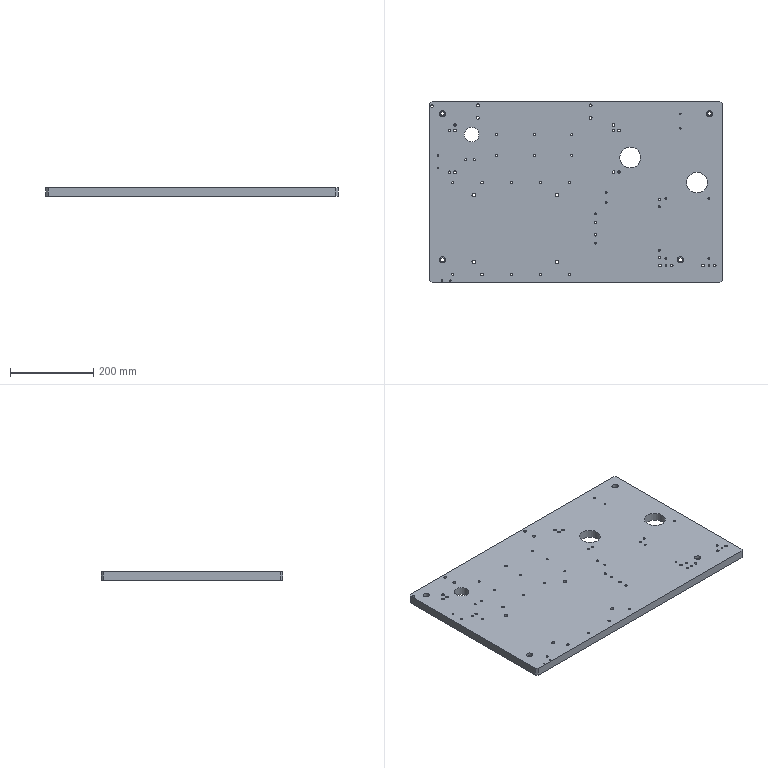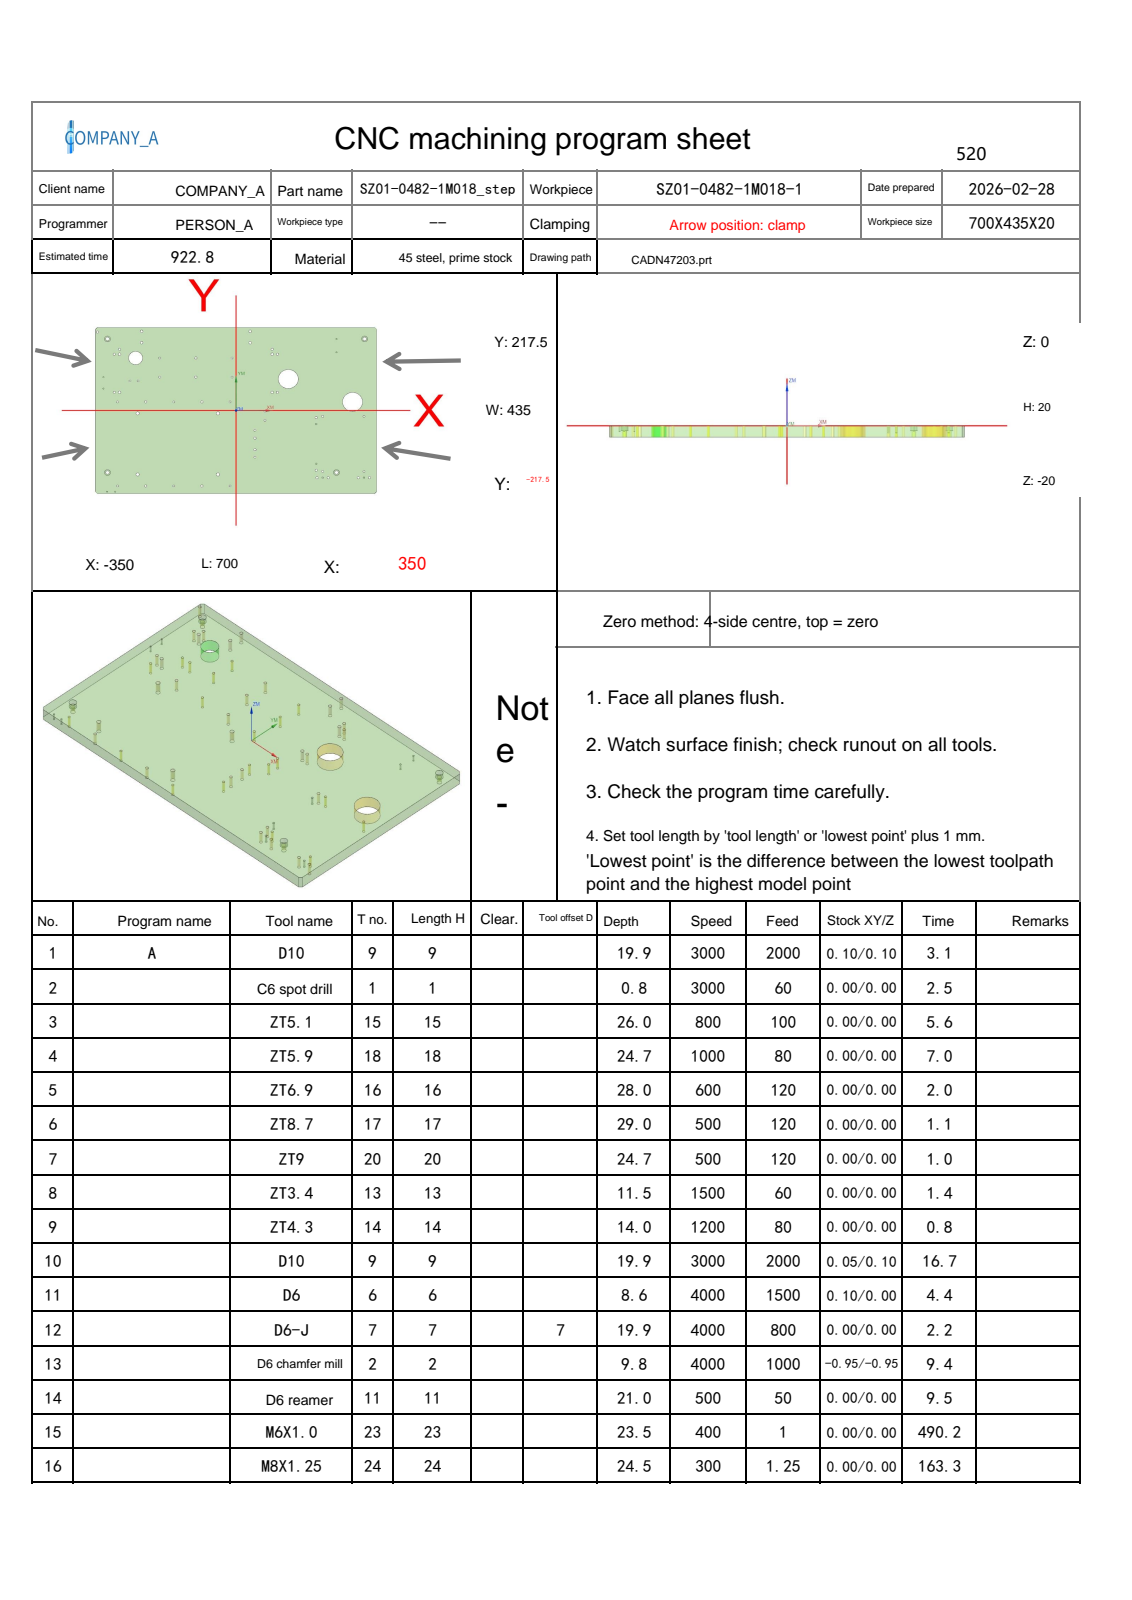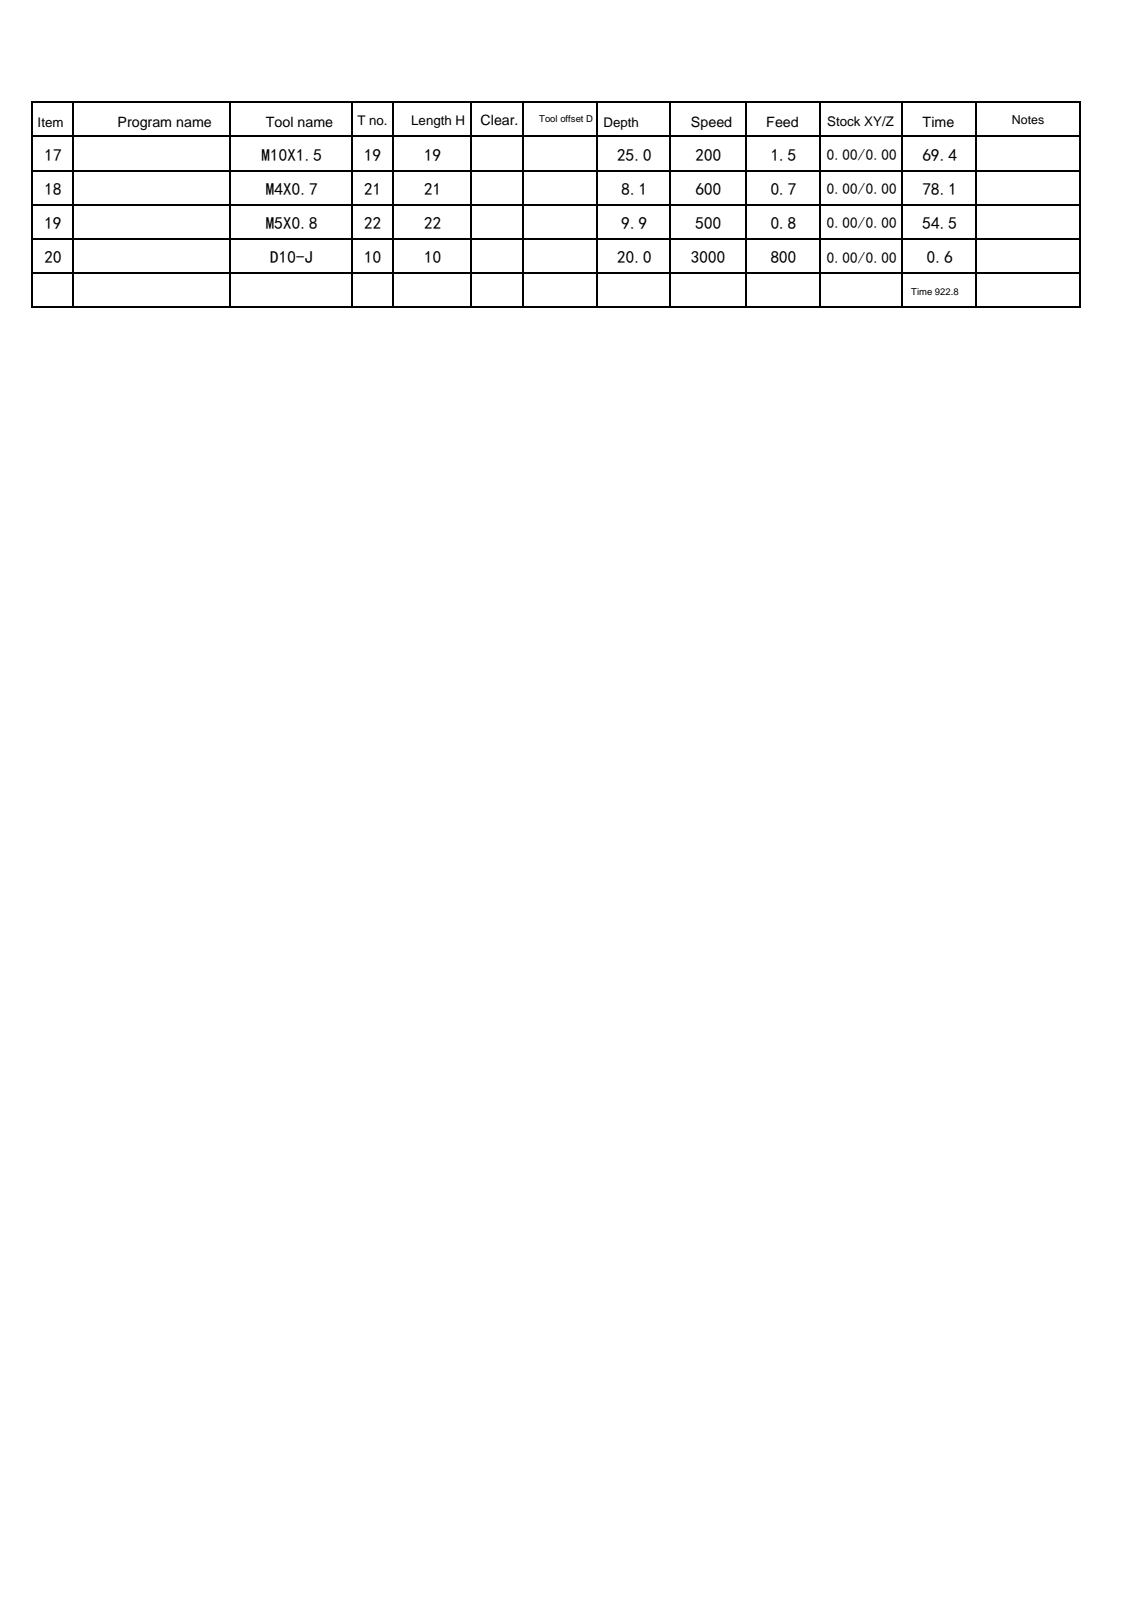NC program | NX | posted by the shop | part box 700 x 435 x 20 mm
Lines 3079 to 5271 of 5271, first 1726 of 2193 lines:
N13 T02 M06
(D6 chamfer mill  D=6. R=0. H=02 ce=0.00 di=0.00)
G00 G90 G54 X250. Y187.5 M03 S4000
G43 H02 Z50.
M08
G98 G81 X250. Y187.5 Z-2.2 R3. F80.
Y152.5
X-330. Y87.5
Y57.5
X-321. Y-212.5
X-301.
G80
G00 Z50.
G00 G90 X318.407 Y-175.306 M03 S4000
Z50.
Z-.5
G01 Z-1. F300.
X318.3 Y-174.5
G03 X316.8 Y-176. I0.0 J-1.5
X318.5 Y-177.7 I1.7 J0.0
X320.2 Y-176. I0.0 J1.7
X318.5 Y-174.3 I-1.7 J0.0
X316.8 Y-176. I0.0 J-1.7
X318.3 Y-177.5 I1.5 J0.0
G01 X318.407 Y-176.694
Z-.5
G00 Z50.
X215.407 Y-175.306
Z-.5
G01 Z-1.
X215.3 Y-174.5
G03 X213.8 Y-176. I0.0 J-1.5
X215.5 Y-177.7 I1.7 J0.0
X217.2 Y-176. I0.0 J1.7
X215.5 Y-174.3 I-1.7 J0.0
X213.8 Y-176. I0.0 J-1.7
X215.3 Y-177.5 I1.5 J0.0
G01 X215.407 Y-176.694
Z-.5
G00 Z50.
X199.407 Y-138.806
Z-.5
G01 Z-1.
X199.3 Y-138.
G03 X197.8 Y-139.5 I0.0 J-1.5
X199.5 Y-141.2 I1.7 J0.0
X201.2 Y-139.5 I0.0 J1.7
X199.5 Y-137.8 I-1.7 J0.0
X197.8 Y-139.5 I0.0 J-1.7
X199.3 Y-141. I1.5 J0.0
G01 X199.407 Y-140.194
Z-.5
G00 Z50.
Y-34.806
Z-.5
G01 Z-1.
X199.3 Y-34.
G03 X197.8 Y-35.5 I0.0 J-1.5
X199.5 Y-37.2 I1.7 J0.0
X201.2 Y-35.5 I0.0 J1.7
X199.5 Y-33.8 I-1.7 J0.0
X197.8 Y-35.5 I0.0 J-1.7
X199.3 Y-37. I1.5 J0.0
G01 X199.407 Y-36.194
Z-.5
G00 Z50.
G00 G90 X-295.409 Y-196.479 M03 S4000
Z50.
Z-.6
G01 Z-1.1 F300.
X-295.6 Y-196.
G03 X-297.1 Y-197.5 I0.0 J-1.5
X-295. Y-199.6 I2.1 J0.0
X-292.9 Y-197.5 I0.0 J2.1
X-295. Y-195.4 I-2.1 J0.0
X-297.1 Y-197.5 I0.0 J-2.1
X-295.6 Y-199. I1.5 J0.0
G01 X-295.409 Y-198.521
Z-.6
G00 Z50.
X-155.409 Y-196.479
Z-.6
G01 Z-1.1
X-155.6 Y-196.
G03 X-157.1 Y-197.5 I0.0 J-1.5
X-155. Y-199.6 I2.1 J0.0
X-152.9 Y-197.5 I0.0 J2.1
X-155. Y-195.4 I-2.1 J0.0
X-157.1 Y-197.5 I0.0 J-2.1
X-155.6 Y-199. I1.5 J0.0
G01 X-155.409 Y-198.521
Z-.6
G00 Z50.
X-15.409 Y-196.479
Z-.6
G01 Z-1.1
X-15.6 Y-196.
G03 X-17.1 Y-197.5 I0.0 J-1.5
X-15. Y-199.6 I2.1 J0.0
X-12.9 Y-197.5 I0.0 J2.1
X-15. Y-195.4 I-2.1 J0.0
X-17.1 Y-197.5 I0.0 J-2.1
X-15.6 Y-199. I1.5 J0.0
G01 X-15.409 Y-198.521
Z-.6
G00 Z50.
X46.591 Y-121.479
Z-.6
G01 Z-1.1
X46.4 Y-121.
G03 X44.9 Y-122.5 I0.0 J-1.5
X47. Y-124.6 I2.1 J0.0
X49.1 Y-122.5 I0.0 J2.1
X47. Y-120.4 I-2.1 J0.0
X44.9 Y-122.5 I0.0 J-2.1
X46.4 Y-124. I1.5 J0.0
G01 X46.591 Y-123.521
Z-.6
G00 Z50.
X215.091 Y-158.479
Z-.6
G01 Z-1.1
X214.9 Y-158.
G03 X213.4 Y-159.5 I0.0 J-1.5
X215.5 Y-161.6 I2.1 J0.0
X217.6 Y-159.5 I0.0 J2.1
X215.5 Y-157.4 I-2.1 J0.0
X213.4 Y-159.5 I0.0 J-2.1
X214.9 Y-161. I1.5 J0.0
G01 X215.091 Y-160.521
Z-.6
G00 Z50.
X318.091 Y-158.479
Z-.6
G01 Z-1.1
X317.9 Y-158.
G03 X316.4 Y-159.5 I0.0 J-1.5
X318.5 Y-161.6 I2.1 J0.0
X320.6 Y-159.5 I0.0 J2.1
X318.5 Y-157.4 I-2.1 J0.0
X316.4 Y-159.5 I0.0 J-2.1
X317.9 Y-161. I1.5 J0.0
G01 X318.091 Y-160.521
Z-.6
G00 Z50.
Y-14.479
Z-.6
G01 Z-1.1
X317.9 Y-14.
G03 X316.4 Y-15.5 I0.0 J-1.5
X318.5 Y-17.6 I2.1 J0.0
X320.6 Y-15.5 I0.0 J2.1
X318.5 Y-13.4 I-2.1 J0.0
X316.4 Y-15.5 I0.0 J-2.1
X317.9 Y-17. I1.5 J0.0
G01 X318.091 Y-16.521
Z-.6
G00 Z50.
X215.091 Y-14.479
Z-.6
G01 Z-1.1
X214.9 Y-14.
G03 X213.4 Y-15.5 I0.0 J-1.5
X215.5 Y-17.6 I2.1 J0.0
X217.6 Y-15.5 I0.0 J2.1
X215.5 Y-13.4 I-2.1 J0.0
X213.4 Y-15.5 I0.0 J-2.1
X214.9 Y-17. I1.5 J0.0
G01 X215.091 Y-16.521
Z-.6
G00 Z50.
X71.591 Y-.479
Z-.6
G01 Z-1.1
X71.4 Y0.0
G03 X69.9 Y-1.5 I0.0 J-1.5
X72. Y-3.6 I2.1 J0.0
X74.1 Y-1.5 I0.0 J2.1
X72. Y.6 I-2.1 J0.0
X69.9 Y-1.5 I0.0 J-2.1
X71.4 Y-3. I1.5 J0.0
G01 X71.591 Y-2.521
Z-.6
G00 Z50.
Y-24.479
Z-.6
G01 Z-1.1
X71.4 Y-24.
G03 X69.9 Y-25.5 I0.0 J-1.5
X72. Y-27.6 I2.1 J0.0
X74.1 Y-25.5 I0.0 J2.1
X72. Y-23.4 I-2.1 J0.0
X69.9 Y-25.5 I0.0 J-2.1
X71.4 Y-27. I1.5 J0.0
G01 X71.591 Y-26.521
Z-.6
G00 Z50.
X46.591 Y-51.479
Z-.6
G01 Z-1.1
X46.4 Y-51.
G03 X44.9 Y-52.5 I0.0 J-1.5
X47. Y-54.6 I2.1 J0.0
X49.1 Y-52.5 I0.0 J2.1
X47. Y-50.4 I-2.1 J0.0
X44.9 Y-52.5 I0.0 J-2.1
X46.4 Y-54. I1.5 J0.0
G01 X46.591 Y-53.521
Z-.6
G00 Z50.
X-15.409 Y23.521
Z-.6
G01 Z-1.1
X-15.6 Y24.
G03 X-17.1 Y22.5 I0.0 J-1.5
X-15. Y20.4 I2.1 J0.0
X-12.9 Y22.5 I0.0 J2.1
X-15. Y24.6 I-2.1 J0.0
X-17.1 Y22.5 I0.0 J-2.1
X-15.6 Y21. I1.5 J0.0
G01 X-15.409 Y21.479
Z-.6
G00 Z50.
X-10.409 Y138.521
Z-.6
G01 Z-1.1
X-10.6 Y139.
G03 X-12.1 Y137.5 I0.0 J-1.5
X-10. Y135.4 I2.1 J0.0
X-7.9 Y137.5 I0.0 J2.1
X-10. Y139.6 I-2.1 J0.0
X-12.1 Y137.5 I0.0 J-2.1
X-10.6 Y136. I1.5 J0.0
G01 X-10.409 Y136.479
Z-.6
G00 Z50.
Y88.521
Z-.6
G01 Z-1.1
X-10.6 Y89.
G03 X-12.1 Y87.5 I0.0 J-1.5
X-10. Y85.4 I2.1 J0.0
X-7.9 Y87.5 I0.0 J2.1
X-10. Y89.6 I-2.1 J0.0
X-12.1 Y87.5 I0.0 J-2.1
X-10.6 Y86. I1.5 J0.0
G01 X-10.409 Y86.479
Z-.6
G00 Z50.
X-155.409 Y23.521
Z-.6
G01 Z-1.1
X-155.6 Y24.
G03 X-157.1 Y22.5 I0.0 J-1.5
X-155. Y20.4 I2.1 J0.0
X-152.9 Y22.5 I0.0 J2.1
X-155. Y24.6 I-2.1 J0.0
X-157.1 Y22.5 I0.0 J-2.1
X-155.6 Y21. I1.5 J0.0
G01 X-155.409 Y21.479
Z-.6
G00 Z50.
X-190.409 Y88.521
Z-.6
G01 Z-1.1
X-190.6 Y89.
G03 X-192.1 Y87.5 I0.0 J-1.5
X-190. Y85.4 I2.1 J0.0
X-187.9 Y87.5 I0.0 J2.1
X-190. Y89.6 I-2.1 J0.0
X-192.1 Y87.5 I0.0 J-2.1
X-190.6 Y86. I1.5 J0.0
G01 X-190.409 Y86.479
Z-.6
G00 Z50.
Y138.521
Z-.6
G01 Z-1.1
X-190.6 Y139.
G03 X-192.1 Y137.5 I0.0 J-1.5
X-190. Y135.4 I2.1 J0.0
X-187.9 Y137.5 I0.0 J2.1
X-190. Y139.6 I-2.1 J0.0
X-192.1 Y137.5 I0.0 J-2.1
X-190.6 Y136. I1.5 J0.0
G01 X-190.409 Y136.479
Z-.6
G00 Z50.
X-244.409 Y78.521
Z-.6
G01 Z-1.1
X-244.6 Y79.
G03 X-246.1 Y77.5 I0.0 J-1.5
X-244. Y75.4 I2.1 J0.0
X-241.9 Y77.5 I0.0 J2.1
X-244. Y79.6 I-2.1 J0.0
X-246.1 Y77.5 I0.0 J-2.1
X-244.6 Y76. I1.5 J0.0
G01 X-244.409 Y76.479
Z-.6
G00 Z50.
X-264.409 Y78.521
Z-.6
G01 Z-1.1
X-264.6 Y79.
G03 X-266.1 Y77.5 I0.0 J-1.5
X-264. Y75.4 I2.1 J0.0
X-261.9 Y77.5 I0.0 J2.1
X-264. Y79.6 I-2.1 J0.0
X-266.1 Y77.5 I0.0 J-2.1
X-264.6 Y76. I1.5 J0.0
G01 X-264.409 Y76.479
Z-.6
G00 Z50.
X-295.409 Y23.521
Z-.6
G01 Z-1.1
X-295.6 Y24.
G03 X-297.1 Y22.5 I0.0 J-1.5
X-295. Y20.4 I2.1 J0.0
X-292.9 Y22.5 I0.0 J2.1
X-295. Y24.6 I-2.1 J0.0
X-297.1 Y22.5 I0.0 J-2.1
X-295.6 Y21. I1.5 J0.0
G01 X-295.409 Y21.479
Z-.6
G00 Z50.
G00 G90 X-345.612 Y206.647 M03 S4000
Z50.
Z-.5
G01 Z-1. F400.
X-345.8 Y207.
G03 X-347.3 Y205.5 I0.0 J-1.5
X-345. Y203.2 I2.3 J0.0
X-342.7 Y205.5 I0.0 J2.3
X-345. Y207.8 I-2.3 J0.0
X-347.3 Y205.5 I0.0 J-2.3
X-345.8 Y204. I1.5 J0.0
G01 X-345.612 Y204.353
Z-.5
G00 Z50.
X-290.612 Y161.647
Z-.5
G01 Z-1.
X-290.8 Y162.
G03 X-292.3 Y160.5 I0.0 J-1.5
X-290. Y158.2 I2.3 J0.0
X-287.7 Y160.5 I0.0 J2.3
X-290. Y162.8 I-2.3 J0.0
X-292.3 Y160.5 I0.0 J-2.3
X-290.8 Y159. I1.5 J0.0
G01 X-290.612 Y159.353
Z-.5
G00 Z50.
X-303.612 Y148.647
Z-.5
G01 Z-1.
X-303.8 Y149.
G03 X-305.3 Y147.5 I0.0 J-1.5
X-303. Y145.2 I2.3 J0.0
X-300.7 Y147.5 I0.0 J2.3
X-303. Y149.8 I-2.3 J0.0
X-305.3 Y147.5 I0.0 J-2.3
X-303.8 Y146. I1.5 J0.0
G01 X-303.612 Y146.353
Z-.5
G00 Z50.
Y48.647
Z-.5
G01 Z-1.
X-303.8 Y49.
G03 X-305.3 Y47.5 I0.0 J-1.5
X-303. Y45.2 I2.3 J0.0
X-300.7 Y47.5 I0.0 J2.3
X-303. Y49.8 I-2.3 J0.0
X-305.3 Y47.5 I0.0 J-2.3
X-303.8 Y46. I1.5 J0.0
G01 X-303.612 Y46.353
Z-.5
G00 Z50.
X-225.612 Y23.647
Z-.5
G01 Z-1.
X-225.8 Y24.
G03 X-227.3 Y22.5 I0.0 J-1.5
X-225. Y20.2 I2.3 J0.0
X-222.7 Y22.5 I0.0 J2.3
X-225. Y24.8 I-2.3 J0.0
X-227.3 Y22.5 I0.0 J-2.3
X-225.8 Y21. I1.5 J0.0
G01 X-225.612 Y21.353
Z-.5
G00 Z50.
X-85.612 Y23.647
Z-.5
G01 Z-1.
X-85.8 Y24.
G03 X-87.3 Y22.5 I0.0 J-1.5
X-85. Y20.2 I2.3 J0.0
X-82.7 Y22.5 I0.0 J2.3
X-85. Y24.8 I-2.3 J0.0
X-87.3 Y22.5 I0.0 J-2.3
X-85.8 Y21. I1.5 J0.0
G01 X-85.612 Y21.353
Z-.5
G00 Z50.
X-100.612 Y88.647
Z-.5
G01 Z-1.
X-100.8 Y89.
G03 X-102.3 Y87.5 I0.0 J-1.5
X-100. Y85.2 I2.3 J0.0
X-97.7 Y87.5 I0.0 J2.3
X-100. Y89.8 I-2.3 J0.0
X-102.3 Y87.5 I0.0 J-2.3
X-100.8 Y86. I1.5 J0.0
G01 X-100.612 Y86.353
Z-.5
G00 Z50.
Y138.647
Z-.5
G01 Z-1.
X-100.8 Y139.
G03 X-102.3 Y137.5 I0.0 J-1.5
X-100. Y135.2 I2.3 J0.0
X-97.7 Y137.5 I0.0 J2.3
X-100. Y139.8 I-2.3 J0.0
X-102.3 Y137.5 I0.0 J-2.3
X-100.8 Y136. I1.5 J0.0
G01 X-100.612 Y136.353
Z-.5
G00 Z50.
X89.388 Y161.647
Z-.5
G01 Z-1.
X89.2 Y162.
G03 X87.7 Y160.5 I0.0 J-1.5
X90. Y158.2 I2.3 J0.0
X92.3 Y160.5 I0.0 J2.3
X90. Y162.8 I-2.3 J0.0
X87.7 Y160.5 I0.0 J-2.3
X89.2 Y159. I1.5 J0.0
G01 X89.388 Y159.353
Z-.5
G00 Z50.
X102.388 Y148.647
Z-.5
G01 Z-1.
X102.2 Y149.
G03 X100.7 Y147.5 I0.0 J-1.5
X103. Y145.2 I2.3 J0.0
X105.3 Y147.5 I0.0 J2.3
X103. Y149.8 I-2.3 J0.0
X100.7 Y147.5 I0.0 J-2.3
X102.2 Y146. I1.5 J0.0
G01 X102.388 Y146.353
Z-.5
G00 Z50.
Y48.647
Z-.5
G01 Z-1.
X102.2 Y49.
G03 X100.7 Y47.5 I0.0 J-1.5
X103. Y45.2 I2.3 J0.0
X105.3 Y47.5 I0.0 J2.3
X103. Y49.8 I-2.3 J0.0
X100.7 Y47.5 I0.0 J-2.3
X102.2 Y46. I1.5 J0.0
G01 X102.388 Y46.353
Z-.5
G00 Z50.
X198.888 Y-17.353
Z-.5
G01 Z-1.
X198.7 Y-17.
G03 X197.2 Y-18.5 I0.0 J-1.5
X199.5 Y-20.8 I2.3 J0.0
X201.8 Y-18.5 I0.0 J2.3
X199.5 Y-16.2 I-2.3 J0.0
X197.2 Y-18.5 I0.0 J-2.3
X198.7 Y-20. I1.5 J0.0
G01 X198.888 Y-19.647
Z-.5
G00 Z50.
Y-155.353
Z-.5
G01 Z-1.
X198.7 Y-155.
G03 X197.2 Y-156.5 I0.0 J-1.5
X199.5 Y-158.8 I2.3 J0.0
X201.8 Y-156.5 I0.0 J2.3
X199.5 Y-154.2 I-2.3 J0.0
X197.2 Y-156.5 I0.0 J-2.3
X198.7 Y-158. I1.5 J0.0
G01 X198.888 Y-157.647
Z-.5
G00 Z50.
X303.888 Y-174.853
Z-.5
G01 Z-1.
X303.7 Y-174.5
G03 X302.2 Y-176. I0.0 J-1.5
X304.5 Y-178.3 I2.3 J0.0
X306.8 Y-176. I0.0 J2.3
X304.5 Y-173.7 I-2.3 J0.0
X302.2 Y-176. I0.0 J-2.3
X303.7 Y-177.5 I1.5 J0.0
G01 X303.888 Y-177.147
Z-.5
G00 Z50.
X331.888 Y-174.853
Z-.5
G01 Z-1.
X331.7 Y-174.5
G03 X330.2 Y-176. I0.0 J-1.5
X332.5 Y-178.3 I2.3 J0.0
X334.8 Y-176. I0.0 J2.3
X332.5 Y-173.7 I-2.3 J0.0
X330.2 Y-176. I0.0 J-2.3
X331.7 Y-177.5 I1.5 J0.0
G01 X331.888 Y-177.147
Z-.5
G00 Z50.
X228.888 Y-174.853
Z-.5
G01 Z-1.
X228.7 Y-174.5
G03 X227.2 Y-176. I0.0 J-1.5
X229.5 Y-178.3 I2.3 J0.0
X231.8 Y-176. I0.0 J2.3
X229.5 Y-173.7 I-2.3 J0.0
X227.2 Y-176. I0.0 J-2.3
X228.7 Y-177.5 I1.5 J0.0
G01 X228.888 Y-177.147
Z-.5
G00 Z50.
X200.888 Y-174.853
Z-.5
G01 Z-1.
X200.7 Y-174.5
G03 X199.2 Y-176. I0.0 J-1.5
X201.5 Y-178.3 I2.3 J0.0
X203.8 Y-176. I0.0 J2.3
X201.5 Y-173.7 I-2.3 J0.0
X199.2 Y-176. I0.0 J-2.3
X200.7 Y-177.5 I1.5 J0.0
G01 X200.888 Y-177.147
Z-.5
G00 Z50.
X46.388 Y-71.353
Z-.5
G01 Z-1.
X46.2 Y-71.
G03 X44.7 Y-72.5 I0.0 J-1.5
X47. Y-74.8 I2.3 J0.0
X49.3 Y-72.5 I0.0 J2.3
X47. Y-70.2 I-2.3 J0.0
X44.7 Y-72.5 I0.0 J-2.3
X46.2 Y-74. I1.5 J0.0
G01 X46.388 Y-73.647
Z-.5
G00 Z50.
Y-101.353
Z-.5
G01 Z-1.
X46.2 Y-101.
G03 X44.7 Y-102.5 I0.0 J-1.5
X47. Y-104.8 I2.3 J0.0
X49.3 Y-102.5 I0.0 J2.3
X47. Y-100.2 I-2.3 J0.0
X44.7 Y-102.5 I0.0 J-2.3
X46.2 Y-104. I1.5 J0.0
G01 X46.388 Y-103.647
Z-.5
G00 Z50.
X-85.612 Y-196.353
Z-.5
G01 Z-1.
X-85.8 Y-196.
G03 X-87.3 Y-197.5 I0.0 J-1.5
X-85. Y-199.8 I2.3 J0.0
X-82.7 Y-197.5 I0.0 J2.3
X-85. Y-195.2 I-2.3 J0.0
X-87.3 Y-197.5 I0.0 J-2.3
X-85.8 Y-199. I1.5 J0.0
G01 X-85.612 Y-198.647
Z-.5
G00 Z50.
X-225.612 Y-196.353
Z-.5
G01 Z-1.
X-225.8 Y-196.
G03 X-227.3 Y-197.5 I0.0 J-1.5
X-225. Y-199.8 I2.3 J0.0
X-222.7 Y-197.5 I0.0 J2.3
X-225. Y-195.2 I-2.3 J0.0
X-227.3 Y-197.5 I0.0 J-2.3
X-225.8 Y-199. I1.5 J0.0
G01 X-225.612 Y-198.647
Z-.5
G00 Z50.
G00 G90 X89.2 Y49. M03 S4000
Z50.
Z-1.
G01 Z-1.5 F500.
X88.8
G03 X87.3 Y47.5 I0.0 J-1.5
X90. Y44.8 I2.7 J0.0
X92.7 Y47.5 I0.0 J2.7
X90. Y50.2 I-2.7 J0.0
X87.3 Y47.5 I0.0 J-2.7
X88.8 Y46. I1.5 J0.0
G01 X89.2
Z-1.
G00 Z50.
Y149.
Z-1.
G01 Z-1.5
X88.8
G03 X87.3 Y147.5 I0.0 J-1.5
X90. Y144.8 I2.7 J0.0
X92.7 Y147.5 I0.0 J2.7
X90. Y150.2 I-2.7 J0.0
X87.3 Y147.5 I0.0 J-2.7
X88.8 Y146. I1.5 J0.0
G01 X89.2
Z-1.
G00 Z50.
X34.2 Y179.
Z-1.
G01 Z-1.5
X33.8
G03 X32.3 Y177.5 I0.0 J-1.5
X35. Y174.8 I2.7 J0.0
X37.7 Y177.5 I0.0 J2.7
X35. Y180.2 I-2.7 J0.0
X32.3 Y177.5 I0.0 J-2.7
X33.8 Y176. I1.5 J0.0
G01 X34.2
Z-1.
G00 Z50.
Y209.
Z-1.
G01 Z-1.5
X33.8
G03 X32.3 Y207.5 I0.0 J-1.5
X35. Y204.8 I2.7 J0.0
X37.7 Y207.5 I0.0 J2.7
X35. Y210.2 I-2.7 J0.0
X32.3 Y207.5 I0.0 J-2.7
X33.8 Y206. I1.5 J0.0
G01 X34.2
Z-1.
G00 Z50.
X-235.8 Y209.
Z-1.
G01 Z-1.5
X-236.2
G03 X-237.7 Y207.5 I0.0 J-1.5
X-235. Y204.8 I2.7 J0.0
X-232.3 Y207.5 I0.0 J2.7
X-235. Y210.2 I-2.7 J0.0
X-237.7 Y207.5 I0.0 J-2.7
X-236.2 Y206. I1.5 J0.0
G01 X-235.8
Z-1.
G00 Z50.
Y179.
Z-1.
G01 Z-1.5
X-236.2
G03 X-237.7 Y177.5 I0.0 J-1.5
X-235. Y174.8 I2.7 J0.0
X-232.3 Y177.5 I0.0 J2.7
X-235. Y180.2 I-2.7 J0.0
X-237.7 Y177.5 I0.0 J-2.7
X-236.2 Y176. I1.5 J0.0
G01 X-235.8
Z-1.
G00 Z50.
X-290.8 Y149.
Z-1.
G01 Z-1.5
X-291.2
G03 X-292.7 Y147.5 I0.0 J-1.5
X-290. Y144.8 I2.7 J0.0
X-287.3 Y147.5 I0.0 J2.7
X-290. Y150.2 I-2.7 J0.0
X-292.7 Y147.5 I0.0 J-2.7
X-291.2 Y146. I1.5 J0.0
G01 X-290.8
Z-1.
G00 Z50.
Y49.
Z-1.
G01 Z-1.5
X-291.2
G03 X-292.7 Y47.5 I0.0 J-1.5
X-290. Y44.8 I2.7 J0.0
X-287.3 Y47.5 I0.0 J2.7
X-290. Y50.2 I-2.7 J0.0
X-292.7 Y47.5 I0.0 J-2.7
X-291.2 Y46. I1.5 J0.0
G01 X-290.8
Z-1.
G00 Z50.
G00 G90 X-45.614 Y-4.871 M03 S4000
Z50.
Z-1.
G01 Z-1.5 F500.
X-45.7 Y-4.5
G03 X-48.7 Y-7.5 I0.0 J-3.
X-45. Y-11.2 I3.7 J0.0
X-41.3 Y-7.5 I0.0 J3.7
X-45. Y-3.8 I-3.7 J0.0
X-48.7 Y-7.5 I0.0 J-3.7
X-45.7 Y-10.5 I3. J0.0
G01 X-45.614 Y-10.129
Z-1.
G00 Z50.
Y-164.871
Z-1.
G01 Z-1.5
X-45.7 Y-164.5
G03 X-48.7 Y-167.5 I0.0 J-3.
X-45. Y-171.2 I3.7 J0.0
X-41.3 Y-167.5 I0.0 J3.7
X-45. Y-163.8 I-3.7 J0.0
X-48.7 Y-167.5 I0.0 J-3.7
X-45.7 Y-170.5 I3. J0.0
G01 X-45.614 Y-170.129
Z-1.
G00 Z50.
X-245.614 Y-164.871
Z-1.
G01 Z-1.5
X-245.7 Y-164.5
G03 X-248.7 Y-167.5 I0.0 J-3.
X-245. Y-171.2 I3.7 J0.0
X-241.3 Y-167.5 I0.0 J3.7
X-245. Y-163.8 I-3.7 J0.0
X-248.7 Y-167.5 I0.0 J-3.7
X-245.7 Y-170.5 I3. J0.0
G01 X-245.614 Y-170.129
Z-1.
G00 Z50.
Y-4.871
Z-1.
G01 Z-1.5
X-245.7 Y-4.5
G03 X-248.7 Y-7.5 I0.0 J-3.
X-245. Y-11.2 I3.7 J0.0
X-241.3 Y-7.5 I0.0 J3.7
X-245. Y-3.8 I-3.7 J0.0
X-248.7 Y-7.5 I0.0 J-3.7
X-245.7 Y-10.5 I3. J0.0
G01 X-245.614 Y-10.129
Z-1.
G00 Z50.
G00 G90 X351.275 Y-212.147 M03 S3500
Z57.5
Z.124
G01 Z-1.2 F1000.
G03 X351.04 Y-212.404 I1.351 J-1.475
G01 X351.004 Y-212.446
X351. Y-212.5
X350.966 Y-212.759
X350.866 Y-213.
X350.707 Y-213.207
X345.707 Y-218.207
X345.5 Y-218.366
X345.259 Y-218.466
X345. Y-218.5
X-345.
X-345.259 Y-218.466
X-345.5 Y-218.366
X-345.707 Y-218.207
X-350.707 Y-213.207
X-350.744 Y-213.167
X-350.797 Y-213.155
G03 X-351.14 Y-213.095 I-.518 J-1.932
G01 Z.113
G00 Z57.5
X-351.275 Y212.147
Z.124
G01 Z-1.2
G03 X-351.04 Y212.404 I-1.351 J1.475
G01 X-351.004 Y212.446
X-351. Y212.5
X-350.966 Y212.759
X-350.866 Y213.
X-350.707 Y213.207
X-345.707 Y218.207
X-345.5 Y218.366
X-345.259 Y218.466
X-345. Y218.5
X345.
X345.259 Y218.466
X345.5 Y218.366
X345.707 Y218.207
X350.707 Y213.207
X350.744 Y213.167
X350.797 Y213.155
G03 X351.14 Y213.095 I.518 J1.932
G01 Z.113
G00 Z57.5
X330.692 Y-175.596
Z.257
G01 Z-1.2
G03 X330.518 Y-175.898 I1.638 J-1.147
G01 X330.492 Y-175.946
X330.5 Y-176.
G03 X332.5 Y-178. I2. J0.0
X334.5 Y-176. I0.0 J2.
X332.5 Y-174. I-2. J0.0
X330.53 Y-175.653 I0.0 J-2.
G01 X330.5 Y-176.
X330.492 Y-176.054
X330.518 Y-176.102
G03 X330.692 Y-176.404 I1.813 J.845
G01 Z.257
G00 Z57.5
X317.185 Y-159.093
Z.284
G01 Z-1.2
G03 X317.016 Y-159.398 I1.658 J-1.118
G01 X316.991 Y-159.446
X317. Y-159.5
G03 X318.5 Y-161. I1.5 J0.0
X320. Y-159.5 I0.0 J1.5
X318.5 Y-158. I-1.5 J0.0
X317. Y-159.5 I0.0 J-1.5
G01 X316.991 Y-159.554
X317.016 Y-159.602
G03 X317.185 Y-159.907 I1.827 J.813
G01 Z.284
G00 Z57.5
X317.574 Y-175.588
Z.32
G01 Z-1.2
G03 X317.414 Y-175.897 I1.687 J-1.075
G01 X317.39 Y-175.946
X317.4 Y-176.
G03 X318.5 Y-177.1 I1.1 J0.0
X319.6 Y-176. I0.0 J1.1
X318.5 Y-174.9 I-1.1 J0.0
X317.4 Y-176. I0.0 J-1.1
G01 X317.39 Y-176.054
X317.414 Y-176.103
G03 X317.574 Y-176.412 I1.848 J.765
G01 Z.32
G00 Z57.5
X302.692 Y-175.596
Z.257
G01 Z-1.2
G03 X302.518 Y-175.898 I1.638 J-1.147
G01 X302.492 Y-175.946
X302.5 Y-176.
G03 X304.5 Y-178. I2. J0.0
X306.5 Y-176. I0.0 J2.
X304.5 Y-174. I-2. J0.0
X302.53 Y-175.653 I0.0 J-2.
G01 X302.5 Y-176.
X302.492 Y-176.054
X302.518 Y-176.102
G03 X302.692 Y-176.404 I1.813 J.845
G01 Z.257
G00 Z57.5
X243.706 Y-162.103
Z.21
G01 Z-1.2
G03 X243.522 Y-162.399 I1.597 J-1.204
G01 X243.494 Y-162.446
X243.5 Y-162.5
G03 X250. Y-169. I6.5 J0.0
X256.5 Y-162.5 I0.0 J6.5
X250. Y-156. I-6.5 J0.0
X243.5 Y-162.5 I0.0 J-6.5
G01 X243.494 Y-162.554
X243.522 Y-162.601
G03 X243.706 Y-162.897 I1.782 J.908
G01 Z.21
G00 Z57.5
X227.692 Y-175.596
Z.257
G01 Z-1.2
G03 X227.518 Y-175.898 I1.638 J-1.147
G01 X227.492 Y-175.946
X227.5 Y-176.
G03 X229.5 Y-178. I2. J0.0
X231.5 Y-176. I0.0 J2.
X229.5 Y-174. I-2. J0.0
X227.53 Y-175.653 I0.0 J-2.
G01 X227.5 Y-176.
X227.492 Y-176.054
X227.518 Y-176.102
G03 X227.692 Y-176.404 I1.813 J.845
G01 Z.257
G00 Z57.5
X214.574 Y-175.588
Z.32
G01 Z-1.2
G03 X214.414 Y-175.897 I1.687 J-1.075
G01 X214.39 Y-175.946
X214.4 Y-176.
G03 X215.5 Y-177.1 I1.1 J0.0
X216.6 Y-176. I0.0 J1.1
X215.5 Y-174.9 I-1.1 J0.0
X214.4 Y-176. I0.0 J-1.1
G01 X214.39 Y-176.054
X214.414 Y-176.103
G03 X214.574 Y-176.412 I1.848 J.765
G01 Z.32
G00 Z57.5
X199.692 Y-175.596
Z.257
G01 Z-1.2
G03 X199.518 Y-175.898 I1.638 J-1.147
G01 X199.492 Y-175.946
X199.5 Y-176.
G03 X201.5 Y-178. I2. J0.0
X203.5 Y-176. I0.0 J2.
X201.5 Y-174. I-2. J0.0
X199.53 Y-175.653 I0.0 J-2.
G01 X199.5 Y-176.
X199.492 Y-176.054
X199.518 Y-176.102
G03 X199.692 Y-176.404 I1.813 J.845
G01 Z.257
G00 Z57.5
X214.185 Y-159.093
Z.284
G01 Z-1.2
G03 X214.016 Y-159.398 I1.658 J-1.118
G01 X213.991 Y-159.446
X214. Y-159.5
G03 X215.5 Y-161. I1.5 J0.0
X217. Y-159.5 I0.0 J1.5
X215.5 Y-158. I-1.5 J0.0
X214. Y-159.5 I0.0 J-1.5
G01 X213.991 Y-159.554
X214.016 Y-159.602
G03 X214.185 Y-159.907 I1.827 J.813
G01 Z.284
G00 Z57.5
X197.692 Y-156.096
Z.257
G01 Z-1.2
G03 X197.518 Y-156.398 I1.638 J-1.147
G01 X197.492 Y-156.446
X197.5 Y-156.5
G03 X199.5 Y-158.5 I2. J0.0
X201.5 Y-156.5 I0.0 J2.
X199.5 Y-154.5 I-2. J0.0
X197.53 Y-156.153 I0.0 J-2.
G01 X197.5 Y-156.5
X197.492 Y-156.554
X197.518 Y-156.602
G03 X197.692 Y-156.904 I1.813 J.845
G01 Z.257
G00 Z57.5
X198.574 Y-139.088
Z.32
G01 Z-1.2
G03 X198.414 Y-139.397 I1.687 J-1.075
G01 X198.39 Y-139.446
X198.4 Y-139.5
G03 X199.5 Y-140.6 I1.1 J0.0
X200.6 Y-139.5 I0.0 J1.1
X199.5 Y-138.4 I-1.1 J0.0
X198.4 Y-139.5 I0.0 J-1.1
G01 X198.39 Y-139.554
X198.414 Y-139.603
G03 X198.574 Y-139.912 I1.848 J.765
G01 Z.32
G00 Z57.5
Y-35.088
Z.32
G01 Z-1.2
G03 X198.414 Y-35.397 I1.687 J-1.075
G01 X198.39 Y-35.446
X198.4 Y-35.5
G03 X199.5 Y-36.6 I1.1 J0.0
X200.6 Y-35.5 I0.0 J1.1
X199.5 Y-34.4 I-1.1 J0.0
X198.4 Y-35.5 I0.0 J-1.1
G01 X198.39 Y-35.554
X198.414 Y-35.603
G03 X198.574 Y-35.912 I1.848 J.765
G01 Z.32
G00 Z57.5
X197.692 Y-18.096
Z.257
G01 Z-1.2
G03 X197.518 Y-18.398 I1.638 J-1.147
G01 X197.492 Y-18.446
X197.5 Y-18.5
G03 X199.5 Y-20.5 I2. J0.0
X201.5 Y-18.5 I0.0 J2.
X199.5 Y-16.5 I-2. J0.0
X197.53 Y-18.153 I0.0 J-2.
G01 X197.5 Y-18.5
X197.492 Y-18.554
X197.518 Y-18.602
G03 X197.692 Y-18.904 I1.813 J.845
G01 Z.257
G00 Z57.5
X214.185 Y-15.093
Z.284
G01 Z-1.2
G03 X214.016 Y-15.398 I1.658 J-1.118
G01 X213.991 Y-15.446
X214. Y-15.5
G03 X215.5 Y-17. I1.5 J0.0
X217. Y-15.5 I0.0 J1.5
X215.5 Y-14. I-1.5 J0.0
X214. Y-15.5 I0.0 J-1.5
G01 X213.991 Y-15.554
X214.016 Y-15.602
G03 X214.185 Y-15.907 I1.827 J.813
G01 Z.284
G00 Z57.5
X317.185 Y-15.093
Z.284
G01 Z-1.2
G03 X317.016 Y-15.398 I1.658 J-1.118
G01 X316.991 Y-15.446
X317. Y-15.5
G03 X318.5 Y-17. I1.5 J0.0
X320. Y-15.5 I0.0 J1.5
X318.5 Y-14. I-1.5 J0.0
X317. Y-15.5 I0.0 J-1.5
G01 X316.991 Y-15.554
X317.016 Y-15.602
G03 X317.185 Y-15.907 I1.827 J.813
G01 Z.284
G00 Z57.5
X266.216 Y22.892
Z.194
G01 Z-1.2
G03 X266.024 Y22.601 I1.567 J-1.243
G01 X265.996 Y22.554
X266. Y22.5
G03 X290. Y-1.5 I24. J0.0
X314. Y22.5 I0.0 J24.
X290. Y46.5 I-24. J0.0
X266. Y22.5 I0.0 J-24.
G01 X265.996 Y22.446
X266.024 Y22.399
G03 X266.216 Y22.108 I1.759 J.952
G01 Z.194
G00 Z57.5
X313.706 Y187.897
Z.21
G01 Z-1.2
G03 X313.522 Y187.601 I1.597 J-1.204
G01 X313.494 Y187.554
X313.5 Y187.5
G03 X320. Y181. I6.5 J0.0
X326.5 Y187.5 I0.0 J6.5
X320. Y194. I-6.5 J0.0
X313.5 Y187.5 I0.0 J-6.5
G01 X313.494 Y187.446
X313.522 Y187.399
G03 X313.706 Y187.103 I1.782 J.908
G01 Z.21
G00 Z57.5
X249.506 Y187.919
Z.405
G01 Z-1.2
G03 X249.359 Y187.603 I1.732 J-1.
G01 X249.338 Y187.553
X249.35 Y187.5
G03 X250. Y186.85 I.65 J0.0
X250.65 Y187.5 I0.0 J.65
X250. Y188.15 I-.65 J0.0
X249.35 Y187.5 I0.0 J-.65
G01 X249.338 Y187.447
X249.359 Y187.397
G03 X249.506 Y187.081 I1.879 J.684
G01 Z.405
G00 Z57.5
Y152.919
Z.405
G01 Z-1.2
G03 X249.359 Y152.603 I1.732 J-1.
G01 X249.338 Y152.553
X249.35 Y152.5
G03 X250. Y151.85 I.65 J0.0
X250.65 Y152.5 I0.0 J.65
X250. Y153.15 I-.65 J0.0
X249.35 Y152.5 I0.0 J-.65
G01 X249.338 Y152.447
X249.359 Y152.397
G03 X249.506 Y152.081 I1.879 J.684
G01 Z.405
G00 Z57.5
X106.216 Y82.892
Z.194
G01 Z-1.2
G03 X106.024 Y82.601 I1.567 J-1.243
G01 X105.996 Y82.554
X106. Y82.5
G03 X130. Y58.5 I24. J0.0
X154. Y82.5 I0.0 J24.
X130. Y106.5 I-24. J0.0
X106. Y82.5 I0.0 J-24.
G01 X105.996 Y82.446
X106.024 Y82.399
G03 X106.216 Y82.108 I1.759 J.952
G01 Z.194
G00 Z57.5
X101.192 Y147.904
Z.257
G01 Z-1.2
G03 X101.018 Y147.602 I1.638 J-1.147
G01 X100.992 Y147.554
X101. Y147.5
G03 X103. Y145.5 I2. J0.0
X105. Y147.5 I0.0 J2.
X103. Y149.5 I-2. J0.0
X101.03 Y147.847 I0.0 J-2.
G01 X101. Y147.5
X100.992 Y147.446
X101.018 Y147.398
G03 X101.192 Y147.096 I1.813 J.845
G01 Z.257
G00 Z57.5
X87.792 Y147.904
Z.252
G01 Z-1.2
G03 X87.618 Y147.602 I1.638 J-1.147
G01 X87.592 Y147.554
X87.6 Y147.5
G03 X90. Y145.1 I2.4 J0.0
X92.4 Y147.5 I0.0 J2.4
X90. Y149.9 I-2.4 J0.0
X87.6 Y147.5 I0.0 J-2.4
G01 X87.592 Y147.446
X87.618 Y147.398
G03 X87.792 Y147.096 I1.813 J.845
G01 Z.252
G00 Z57.5
X88.192 Y160.904
Z.257
G01 Z-1.2
G03 X88.018 Y160.602 I1.638 J-1.147
G01 X87.992 Y160.554
X88. Y160.5
G03 X90. Y158.5 I2. J0.0
X92. Y160.5 I0.0 J2.
X90. Y162.5 I-2. J0.0
X88.03 Y160.847 I0.0 J-2.
G01 X88. Y160.5
X87.992 Y160.446
X88.018 Y160.398
G03 X88.192 Y160.096 I1.813 J.845
G01 Z.257
G00 Z57.5
X32.792 Y207.904
Z.252
G01 Z-1.2
G03 X32.618 Y207.602 I1.638 J-1.147
G01 X32.592 Y207.554
X32.6 Y207.5
G03 X35. Y205.1 I2.4 J0.0
X37.4 Y207.5 I0.0 J2.4
X35. Y209.9 I-2.4 J0.0
X32.6 Y207.5 I0.0 J-2.4
G01 X32.592 Y207.446
X32.618 Y207.398
G03 X32.792 Y207.096 I1.813 J.845
G01 Z.252
G00 Z57.5
Y177.904
Z.252
G01 Z-1.2
G03 X32.618 Y177.602 I1.638 J-1.147
G01 X32.592 Y177.554
X32.6 Y177.5
G03 X35. Y175.1 I2.4 J0.0
X37.4 Y177.5 I0.0 J2.4
X35. Y179.9 I-2.4 J0.0
X32.6 Y177.5 I0.0 J-2.4
G01 X32.592 Y177.446
X32.618 Y177.398
G03 X32.792 Y177.096 I1.813 J.845
G01 Z.252
G00 Z57.5
X-11.315 Y137.907
Z.284
G01 Z-1.2
G03 X-11.484 Y137.602 I1.658 J-1.118
G01 X-11.509 Y137.554
X-11.5 Y137.5
G03 X-10. Y136. I1.5 J0.0
X-8.5 Y137.5 I0.0 J1.5
X-10. Y139. I-1.5 J0.0
X-11.5 Y137.5 I0.0 J-1.5
G01 X-11.509 Y137.446
X-11.484 Y137.398
G03 X-11.315 Y137.093 I1.827 J.813
G01 Z.284
G00 Z57.5
Y87.907
Z.284
G01 Z-1.2
G03 X-11.484 Y87.602 I1.658 J-1.118
G01 X-11.509 Y87.554
X-11.5 Y87.5
G03 X-10. Y86. I1.5 J0.0
X-8.5 Y87.5 I0.0 J1.5
X-10. Y89. I-1.5 J0.0
X-11.5 Y87.5 I0.0 J-1.5
G01 X-11.509 Y87.446
X-11.484 Y87.398
G03 X-11.315 Y87.093 I1.827 J.813
G01 Z.284
G00 Z57.5
X-101.808 Y87.904
Z.257
G01 Z-1.2
G03 X-101.982 Y87.602 I1.638 J-1.147
G01 X-102.008 Y87.554
X-102. Y87.5
G03 X-100. Y85.5 I2. J0.0
X-98. Y87.5 I0.0 J2.
X-100. Y89.5 I-2. J0.0
X-101.97 Y87.847 I0.0 J-2.
G01 X-102. Y87.5
X-102.008 Y87.446
X-101.982 Y87.398
G03 X-101.808 Y87.096 I1.813 J.845
G01 Z.257
G00 Z57.5
Y137.904
Z.257
G01 Z-1.2
G03 X-101.982 Y137.602 I1.638 J-1.147
G01 X-102.008 Y137.554
X-102. Y137.5
G03 X-100. Y135.5 I2. J0.0
X-98. Y137.5 I0.0 J2.
X-100. Y139.5 I-2. J0.0
X-101.97 Y137.847 I0.0 J-2.
G01 X-102. Y137.5
X-102.008 Y137.446
X-101.982 Y137.398
G03 X-101.808 Y137.096 I1.813 J.845
G01 Z.257
G00 Z57.5
X-191.315 Y137.907
Z.284
G01 Z-1.2
G03 X-191.484 Y137.602 I1.658 J-1.118
G01 X-191.509 Y137.554
X-191.5 Y137.5
G03 X-190. Y136. I1.5 J0.0
X-188.5 Y137.5 I0.0 J1.5
X-190. Y139. I-1.5 J0.0
X-191.5 Y137.5 I0.0 J-1.5
G01 X-191.509 Y137.446
X-191.484 Y137.398
G03 X-191.315 Y137.093 I1.827 J.813
G01 Z.284
G00 Z57.5
X-266.286 Y137.893
Z.195
G01 Z-1.2
G03 X-266.476 Y137.601 I1.573 J-1.235
G01 X-266.505 Y137.554
X-266.5 Y137.5
G03 X-250. Y121. I16.5 J0.0
X-233.5 Y137.5 I0.0 J16.5
X-250. Y154. I-16.5 J0.0
X-266.5 Y137.5 I0.0 J-16.5
G01 X-266.505 Y137.446
X-266.476 Y137.399
G03 X-266.286 Y137.107 I1.764 J.943
G01 Z.195
G00 Z57.5
X-237.208 Y177.904
Z.252
G01 Z-1.2
G03 X-237.382 Y177.602 I1.638 J-1.147
G01 X-237.408 Y177.554
X-237.4 Y177.5
G03 X-235. Y175.1 I2.4 J0.0
X-232.6 Y177.5 I0.0 J2.4
X-235. Y179.9 I-2.4 J0.0
X-237.4 Y177.5 I0.0 J-2.4
G01 X-237.408 Y177.446
X-237.382 Y177.398
G03 X-237.208 Y177.096 I1.813 J.845
G01 Z.252
G00 Z57.5
Y207.904
Z.252
G01 Z-1.2
G03 X-237.382 Y207.602 I1.638 J-1.147
G01 X-237.408 Y207.554
X-237.4 Y207.5
G03 X-235. Y205.1 I2.4 J0.0
X-232.6 Y207.5 I0.0 J2.4
X-235. Y209.9 I-2.4 J0.0
X-237.4 Y207.5 I0.0 J-2.4
G01 X-237.408 Y207.446
X-237.382 Y207.398
G03 X-237.208 Y207.096 I1.813 J.845
G01 Z.252
G00 Z57.5
X-346.808 Y205.904
Z.257
G01 Z-1.2
G03 X-346.982 Y205.602 I1.638 J-1.147
G01 X-347.008 Y205.554
X-347. Y205.5
G03 X-345. Y203.5 I2. J0.0
X-343. Y205.5 I0.0 J2.
X-345. Y207.5 I-2. J0.0
X-346.97 Y205.847 I0.0 J-2.
G01 X-347. Y205.5
X-347.008 Y205.446
X-346.982 Y205.398
G03 X-346.808 Y205.096 I1.813 J.845
G01 Z.257
G00 Z57.5
X-326.294 Y187.897
Z.21
G01 Z-1.2
G03 X-326.478 Y187.601 I1.597 J-1.204
G01 X-326.506 Y187.554
X-326.5 Y187.5
G03 X-320. Y181. I6.5 J0.0
X-313.5 Y187.5 I0.0 J6.5
X-320. Y194. I-6.5 J0.0
X-326.5 Y187.5 I0.0 J-6.5
G01 X-326.506 Y187.446
X-326.478 Y187.399
G03 X-326.294 Y187.103 I1.782 J.908
G01 Z.21
G00 Z57.5
X-291.808 Y160.904
Z.257
G01 Z-1.2
G03 X-291.982 Y160.602 I1.638 J-1.147
G01 X-292.008 Y160.554
X-292. Y160.5
G03 X-290. Y158.5 I2. J0.0
X-288. Y160.5 I0.0 J2.
X-290. Y162.5 I-2. J0.0
X-291.97 Y160.847 I0.0 J-2.
G01 X-292. Y160.5
X-292.008 Y160.446
X-291.982 Y160.398
G03 X-291.808 Y160.096 I1.813 J.845
G01 Z.257
G00 Z57.5
X-292.208 Y147.904
Z.252
G01 Z-1.2
G03 X-292.382 Y147.602 I1.638 J-1.147
G01 X-292.408 Y147.554
X-292.4 Y147.5
G03 X-290. Y145.1 I2.4 J0.0
X-287.6 Y147.5 I0.0 J2.4
X-290. Y149.9 I-2.4 J0.0
X-292.4 Y147.5 I0.0 J-2.4
G01 X-292.408 Y147.446
X-292.382 Y147.398
G03 X-292.208 Y147.096 I1.813 J.845
G01 Z.252
G00 Z57.5
X-304.808 Y147.904
Z.257
G01 Z-1.2
G03 X-304.982 Y147.602 I1.638 J-1.147
G01 X-305.008 Y147.554
X-305. Y147.5
G03 X-303. Y145.5 I2. J0.0
X-301. Y147.5 I0.0 J2.
X-303. Y149.5 I-2. J0.0
X-304.97 Y147.847 I0.0 J-2.
G01 X-305. Y147.5
X-305.008 Y147.446
X-304.982 Y147.398
G03 X-304.808 Y147.096 I1.813 J.845
G01 Z.257
G00 Z57.5
X-330.494 Y87.919
Z.405
G01 Z-1.2
G03 X-330.641 Y87.603 I1.732 J-1.
G01 X-330.662 Y87.553
X-330.65 Y87.5
G03 X-330. Y86.85 I.65 J0.0
X-329.35 Y87.5 I0.0 J.65
X-330. Y88.15 I-.65 J0.0
X-330.65 Y87.5 I0.0 J-.65
G01 X-330.662 Y87.447
X-330.641 Y87.397
G03 X-330.494 Y87.081 I1.879 J.684
G01 Z.405
G00 Z57.5
Y57.919
Z.405
G01 Z-1.2
G03 X-330.641 Y57.603 I1.732 J-1.
G01 X-330.662 Y57.553
X-330.65 Y57.5
G03 X-330. Y56.85 I.65 J0.0
X-329.35 Y57.5 I0.0 J.65
X-330. Y58.15 I-.65 J0.0
X-330.65 Y57.5 I0.0 J-.65
G01 X-330.662 Y57.447
X-330.641 Y57.397
G03 X-330.494 Y57.081 I1.879 J.684
G01 Z.405
G00 Z57.5
X-304.808 Y47.904
Z.257
G01 Z-1.2
G03 X-304.982 Y47.602 I1.638 J-1.147
G01 X-305.008 Y47.554
X-305. Y47.5
G03 X-303. Y45.5 I2. J0.0
X-301. Y47.5 I0.0 J2.
X-303. Y49.5 I-2. J0.0
X-304.97 Y47.847 I0.0 J-2.
G01 X-305. Y47.5
X-305.008 Y47.446
X-304.982 Y47.398
G03 X-304.808 Y47.096 I1.813 J.845
G01 Z.257
G00 Z57.5
X-292.208 Y47.904
Z.252
G01 Z-1.2
G03 X-292.382 Y47.602 I1.638 J-1.147
G01 X-292.408 Y47.554
X-292.4 Y47.5
G03 X-290. Y45.1 I2.4 J0.0
X-287.6 Y47.5 I0.0 J2.4
X-290. Y49.9 I-2.4 J0.0
X-292.4 Y47.5 I0.0 J-2.4
G01 X-292.408 Y47.446
X-292.382 Y47.398
G03 X-292.208 Y47.096 I1.813 J.845
G01 Z.252
G00 Z57.5
X-296.315 Y22.907
Z.284
G01 Z-1.2
G03 X-296.484 Y22.602 I1.658 J-1.118
G01 X-296.509 Y22.554
X-296.5 Y22.5
G03 X-295. Y21. I1.5 J0.0
X-293.5 Y22.5 I0.0 J1.5
X-295. Y24. I-1.5 J0.0
X-296.5 Y22.5 I0.0 J-1.5
G01 X-296.509 Y22.446
X-296.484 Y22.398
G03 X-296.315 Y22.093 I1.827 J.813
G01 Z.284
G00 Z57.5
X-248.053 Y-7.099
Z.232
G01 Z-1.2
G03 X-248.231 Y-7.398 I1.624 J-1.167
G01 X-248.257 Y-7.446
X-248.25 Y-7.5
G03 X-245. Y-10.75 I3.25 J0.0
X-241.75 Y-7.5 I0.0 J3.25
X-245. Y-4.25 I-3.25 J0.0
X-248.25 Y-7.5 I0.0 J-3.25
G01 X-248.257 Y-7.554
X-248.231 Y-7.602
G03 X-248.053 Y-7.901 I1.802 J.868
G01 Z.232
G00 Z57.5
X-226.808 Y22.904
Z.257
G01 Z-1.2
G03 X-226.982 Y22.602 I1.638 J-1.147
G01 X-227.008 Y22.554
X-227. Y22.5
G03 X-225. Y20.5 I2. J0.0
X-223. Y22.5 I0.0 J2.
X-225. Y24.5 I-2. J0.0
X-226.97 Y22.847 I0.0 J-2.
G01 X-227. Y22.5
X-227.008 Y22.446
X-226.982 Y22.398
G03 X-226.808 Y22.096 I1.813 J.845
G01 Z.257
G00 Z57.5
X-265.315 Y77.907
Z.284
G01 Z-1.2
G03 X-265.484 Y77.602 I1.658 J-1.118
G01 X-265.509 Y77.554
X-265.5 Y77.5
G03 X-264. Y76. I1.5 J0.0
X-262.5 Y77.5 I0.0 J1.5
X-264. Y79. I-1.5 J0.0
X-265.5 Y77.5 I0.0 J-1.5
G01 X-265.509 Y77.446
X-265.484 Y77.398
G03 X-265.315 Y77.093 I1.827 J.813
G01 Z.284
G00 Z57.5
X-245.315 Y77.907
Z.284
G01 Z-1.2
G03 X-245.484 Y77.602 I1.658 J-1.118
G01 X-245.509 Y77.554
X-245.5 Y77.5
G03 X-244. Y76. I1.5 J0.0
X-242.5 Y77.5 I0.0 J1.5
X-244. Y79. I-1.5 J0.0
X-245.5 Y77.5 I0.0 J-1.5
G01 X-245.509 Y77.446
X-245.484 Y77.398
G03 X-245.315 Y77.093 I1.827 J.813
G01 Z.284
G00 Z57.5
X-191.315 Y87.907
Z.284
G01 Z-1.2
G03 X-191.484 Y87.602 I1.658 J-1.118
G01 X-191.509 Y87.554
X-191.5 Y87.5
G03 X-190. Y86. I1.5 J0.0
X-188.5 Y87.5 I0.0 J1.5
X-190. Y89. I-1.5 J0.0
X-191.5 Y87.5 I0.0 J-1.5
G01 X-191.509 Y87.446
X-191.484 Y87.398
G03 X-191.315 Y87.093 I1.827 J.813
G01 Z.284
G00 Z57.5
X-156.315 Y22.907
Z.284
G01 Z-1.2
G03 X-156.484 Y22.602 I1.658 J-1.118
G01 X-156.509 Y22.554
X-156.5 Y22.5
G03 X-155. Y21. I1.5 J0.0
X-153.5 Y22.5 I0.0 J1.5
X-155. Y24. I-1.5 J0.0
X-156.5 Y22.5 I0.0 J-1.5
G01 X-156.509 Y22.446
X-156.484 Y22.398
G03 X-156.315 Y22.093 I1.827 J.813
G01 Z.284
G00 Z57.5
X-86.808 Y22.904
Z.257
G01 Z-1.2
G03 X-86.982 Y22.602 I1.638 J-1.147
G01 X-87.008 Y22.554
X-87. Y22.5
G03 X-85. Y20.5 I2. J0.0
X-83. Y22.5 I0.0 J2.
X-85. Y24.5 I-2. J0.0
X-86.97 Y22.847 I0.0 J-2.
G01 X-87. Y22.5
X-87.008 Y22.446
X-86.982 Y22.398
G03 X-86.808 Y22.096 I1.813 J.845
G01 Z.257
G00 Z57.5
X-48.053 Y-7.099
Z.232
G01 Z-1.2
G03 X-48.231 Y-7.398 I1.624 J-1.167
G01 X-48.257 Y-7.446
X-48.25 Y-7.5
G03 X-45. Y-10.75 I3.25 J0.0
X-41.75 Y-7.5 I0.0 J3.25
X-45. Y-4.25 I-3.25 J0.0
X-48.25 Y-7.5 I0.0 J-3.25
G01 X-48.257 Y-7.554
X-48.231 Y-7.602
G03 X-48.053 Y-7.901 I1.802 J.868
G01 Z.232
G00 Z57.5
X-16.315 Y22.907
Z.284
G01 Z-1.2
G03 X-16.484 Y22.602 I1.658 J-1.118
G01 X-16.509 Y22.554
X-16.5 Y22.5
G03 X-15. Y21. I1.5 J0.0
X-13.5 Y22.5 I0.0 J1.5
X-15. Y24. I-1.5 J0.0
X-16.5 Y22.5 I0.0 J-1.5
G01 X-16.509 Y22.446
X-16.484 Y22.398
G03 X-16.315 Y22.093 I1.827 J.813
G01 Z.284
G00 Z57.5
X87.792 Y47.904
Z.252
G01 Z-1.2
G03 X87.618 Y47.602 I1.638 J-1.147
G01 X87.592 Y47.554
X87.6 Y47.5
G03 X90. Y45.1 I2.4 J0.0
X92.4 Y47.5 I0.0 J2.4
X90. Y49.9 I-2.4 J0.0
X87.6 Y47.5 I0.0 J-2.4
G01 X87.592 Y47.446
X87.618 Y47.398
G03 X87.792 Y47.096 I1.813 J.845
G01 Z.252
G00 Z57.5
X101.192 Y47.904
Z.257
G01 Z-1.2
G03 X101.018 Y47.602 I1.638 J-1.147
G01 X100.992 Y47.554
X101. Y47.5
G03 X103. Y45.5 I2. J0.0
X105. Y47.5 I0.0 J2.
X103. Y49.5 I-2. J0.0
X101.03 Y47.847 I0.0 J-2.
G01 X101. Y47.5
X100.992 Y47.446
X101.018 Y47.398
G03 X101.192 Y47.096 I1.813 J.845
G01 Z.257
G00 Z57.5
X70.685 Y-1.093
Z.284
G01 Z-1.2
G03 X70.516 Y-1.398 I1.658 J-1.118
G01 X70.491 Y-1.446
X70.5 Y-1.5
G03 X72. Y-3. I1.5 J0.0
X73.5 Y-1.5 I0.0 J1.5
X72. Y0.0 I-1.5 J0.0
X70.5 Y-1.5 I0.0 J-1.5
G01 X70.491 Y-1.554
X70.516 Y-1.602
G03 X70.685 Y-1.907 I1.827 J.813
G01 Z.284
G00 Z57.5
Y-25.093
Z.284
G01 Z-1.2
G03 X70.516 Y-25.398 I1.658 J-1.118
G01 X70.491 Y-25.446
X70.5 Y-25.5
G03 X72. Y-27. I1.5 J0.0
X73.5 Y-25.5 I0.0 J1.5
X72. Y-24. I-1.5 J0.0
X70.5 Y-25.5 I0.0 J-1.5
G01 X70.491 Y-25.554
X70.516 Y-25.602
G03 X70.685 Y-25.907 I1.827 J.813
G01 Z.284
G00 Z57.5
X45.685 Y-52.093
Z.284
G01 Z-1.2
G03 X45.516 Y-52.398 I1.658 J-1.118
G01 X45.491 Y-52.446
X45.5 Y-52.5
G03 X47. Y-54. I1.5 J0.0
X48.5 Y-52.5 I0.0 J1.5
X47. Y-51. I-1.5 J0.0
X45.5 Y-52.5 I0.0 J-1.5
G01 X45.491 Y-52.554
X45.516 Y-52.602
G03 X45.685 Y-52.907 I1.827 J.813
G01 Z.284
G00 Z57.5
X45.192 Y-72.096
Z.257
G01 Z-1.2
G03 X45.018 Y-72.398 I1.638 J-1.147
G01 X44.992 Y-72.446
X45. Y-72.5
G03 X47. Y-74.5 I2. J0.0
X49. Y-72.5 I0.0 J2.
X47. Y-70.5 I-2. J0.0
X45.03 Y-72.153 I0.0 J-2.
G01 X45. Y-72.5
X44.992 Y-72.554
X45.018 Y-72.602
G03 X45.192 Y-72.904 I1.813 J.845
G01 Z.257
G00 Z57.5
Y-102.096
Z.257
G01 Z-1.2
G03 X45.018 Y-102.398 I1.638 J-1.147
G01 X44.992 Y-102.446
X45. Y-102.5
G03 X47. Y-104.5 I2. J0.0
X49. Y-102.5 I0.0 J2.
X47. Y-100.5 I-2. J0.0
X45.03 Y-102.153 I0.0 J-2.
G01 X45. Y-102.5
X44.992 Y-102.554
X45.018 Y-102.602
G03 X45.192 Y-102.904 I1.813 J.845
G01 Z.257
G00 Z57.5
X45.685 Y-122.093
Z.284
G01 Z-1.2
G03 X45.516 Y-122.398 I1.658 J-1.118
G01 X45.491 Y-122.446
X45.5 Y-122.5
G03 X47. Y-124. I1.5 J0.0
X48.5 Y-122.5 I0.0 J1.5
X47. Y-121. I-1.5 J0.0
X45.5 Y-122.5 I0.0 J-1.5
G01 X45.491 Y-122.554
X45.516 Y-122.602
G03 X45.685 Y-122.907 I1.827 J.813
G01 Z.284
G00 Z57.5
X-16.315 Y-197.093